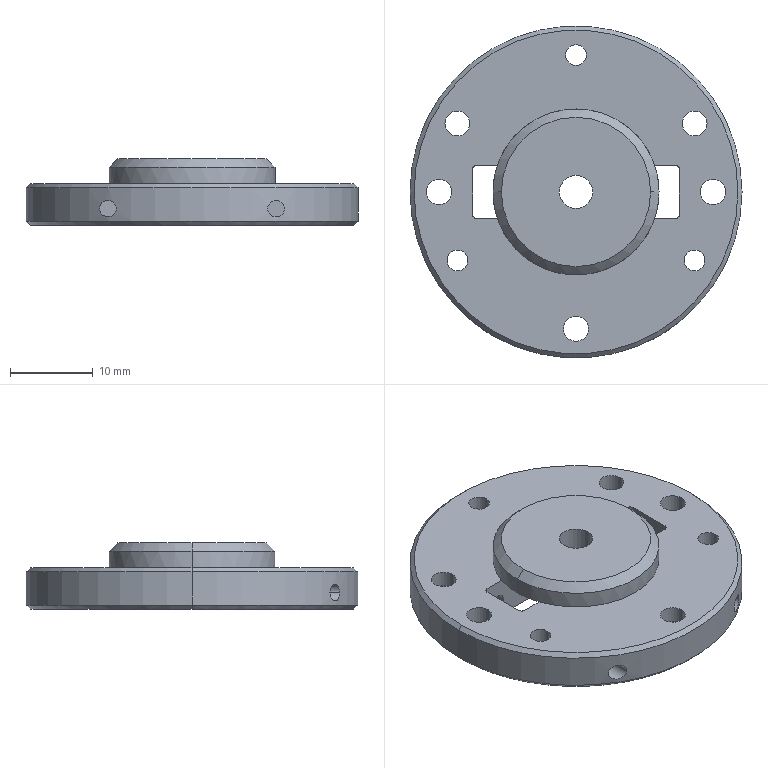Part | NX | features BREP 1 | 1 solid | 63 faces | box 40 x 40 x 8 mm | volume 5675 mm3 | cylinder 42 | plane 15 | cone 6 | commonest cylinder face diameters 2 x8 2.5 x6 3 x6 6 x6 1 x4 3.05 x4